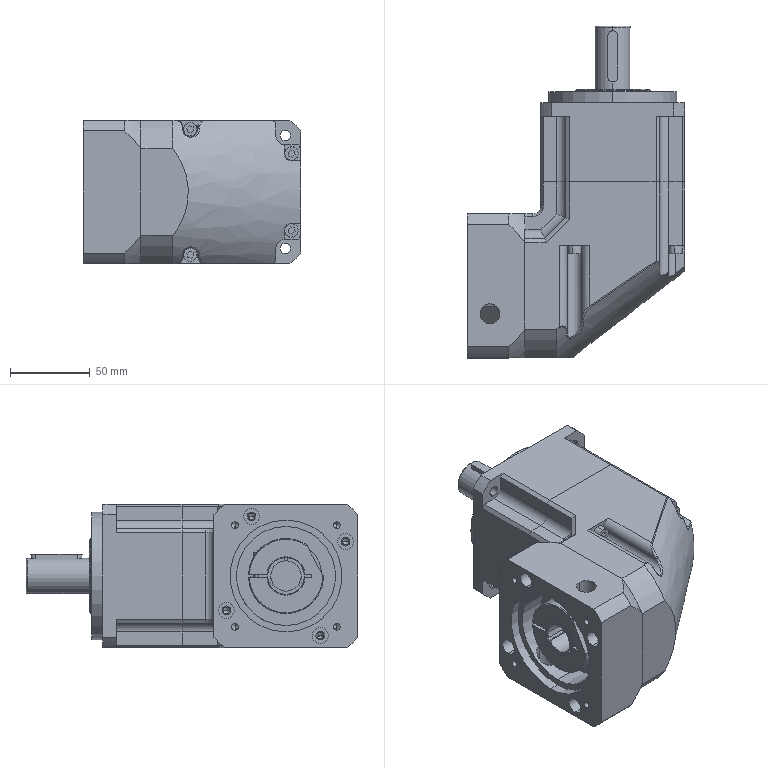Part | SolidWorks | 12 solids | 491 faces | box 136 x 207.5 x 90 mm | volume 1300717 mm3 | cylinder 199 | plane 167 | torus 58 | cone 52 | spline 15 | commonest cylinder face diameters 105 x24 4.2 x16 5 x16 11 x15 8.5 x12 4 x8